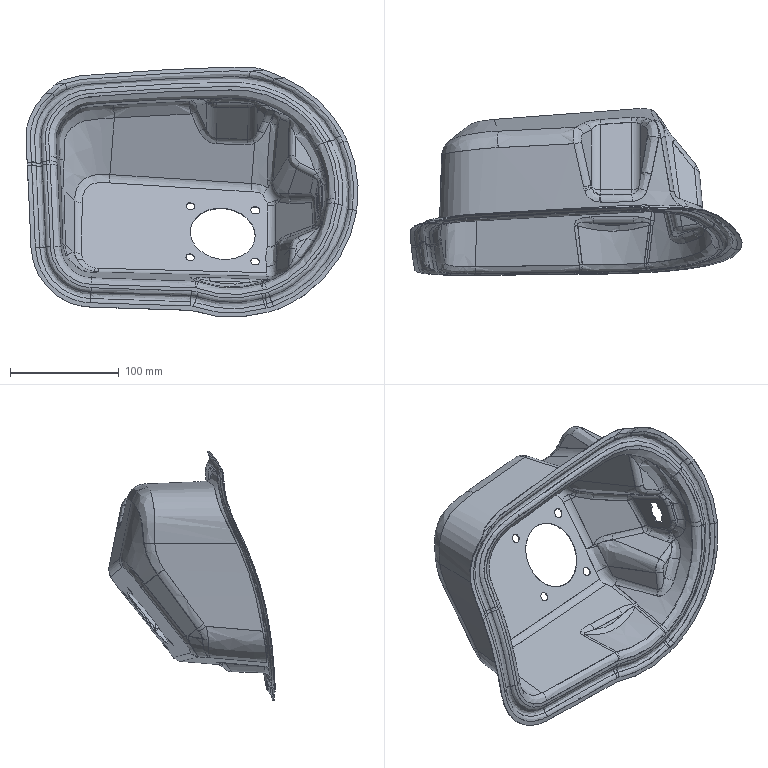Part | STEP file | FNA5401101 | 1 solid | 460 faces | box 305.711 x 153.486 x 230.44 mm | volume 76829 mm3 | spline 366 | cylinder 66 | plane 20 | other 4 | sphere 4 | commonest cylinder face diameters 2 x12 20 x9 16 x7 10 x6 11.4 x6 14.6 x6